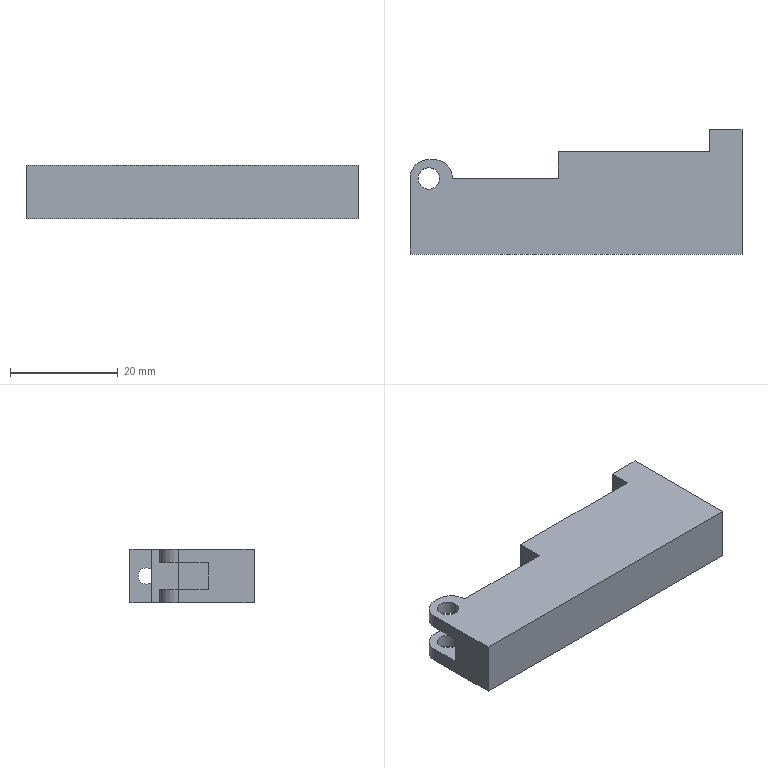Part | SolidWorks | features ICE 2, Extrusion 1 | 1 solid | 25 faces | box 61.5 x 23 x 10 mm | volume 10198 mm3 | plane 15 | cylinder 10 | commonest cylinder face diameters 4 x4 7 x4 3 x2
STEP:
#1=CARTESIAN_POINT('',(0.9754,7.251,6.5));
#2=VERTEX_POINT('',#1);
#3=CARTESIAN_POINT('',(0.9754,6.251,6.118));
#4=VERTEX_POINT('',#3);
#5=CARTESIAN_POINT('',(0.9754,7.251,5.));
#6=DIRECTION('',(1.,0.,0.));
#7=DIRECTION('',(0.,0.,-1.));
#8=AXIS2_PLACEMENT_3D('',#5,#6,#7);
#9=CIRCLE('',#8,1.5);
#10=EDGE_CURVE('',#2,#4,#9,.T.);
#11=ORIENTED_EDGE('',*,*,#10,.F.);
#12=CARTESIAN_POINT('',(6.975,7.251,6.5));
#13=VERTEX_POINT('',#12);
#14=CARTESIAN_POINT('',(0.9754,7.251,6.5));
#15=DIRECTION('',(1.,0.,0.));
#16=VECTOR('',#15,1000.);
#17=LINE('',#14,#16);
#18=EDGE_CURVE('',#2,#13,#17,.T.);
#19=ORIENTED_EDGE('',*,*,#18,.T.);
#20=CARTESIAN_POINT('',(6.975,7.251,3.5));
#21=VERTEX_POINT('',#20);
#22=CARTESIAN_POINT('',(6.975,7.251,5.));
#23=DIRECTION('',(1.,0.,0.));
#24=DIRECTION('',(0.,0.,-1.));
#25=AXIS2_PLACEMENT_3D('',#22,#23,#24);
#26=CIRCLE('',#25,1.5);
#27=EDGE_CURVE('',#13,#21,#26,.T.);
#28=ORIENTED_EDGE('',*,*,#27,.T.);
#29=CARTESIAN_POINT('',(0.9754,7.251,3.5));
#30=VERTEX_POINT('',#29);
#31=CARTESIAN_POINT('',(0.9754,7.251,3.5));
#32=DIRECTION('',(1.,0.,0.));
#33=VECTOR('',#32,1000.);
#34=LINE('',#31,#33);
#35=EDGE_CURVE('',#30,#21,#34,.T.);
#36=ORIENTED_EDGE('',*,*,#35,.F.);
#37=CARTESIAN_POINT('',(0.9754,6.251,3.882));
#38=VERTEX_POINT('',#37);
#39=CARTESIAN_POINT('',(0.9754,7.251,5.));
#40=DIRECTION('',(1.,0.,0.));
#41=DIRECTION('',(0.,0.,-1.));
#42=AXIS2_PLACEMENT_3D('',#39,#40,#41);
#43=CIRCLE('',#42,1.5);
#44=EDGE_CURVE('',#38,#30,#43,.T.);
#45=ORIENTED_EDGE('',*,*,#44,.F.);
#46=CARTESIAN_POINT('',(0.9754,7.251,5.));
#47=DIRECTION('',(1.,0.,0.));
#48=DIRECTION('',(0.,0.,-1.));
#49=AXIS2_PLACEMENT_3D('',#46,#47,#48);
#50=CIRCLE('',#49,1.5);
#51=EDGE_CURVE('',#4,#38,#50,.T.);
#52=ORIENTED_EDGE('',*,*,#51,.F.);
#53=EDGE_LOOP('',(#11,#19,#28,#36,#45,#52));
#54=FACE_OUTER_BOUND('',#53,.T.);
#55=CARTESIAN_POINT('',(0.9754,7.251,5.));
#56=DIRECTION('',(1.,0.,0.));
#57=DIRECTION('',(0.,0.,-1.));
#58=AXIS2_PLACEMENT_3D('',#55,#56,#57);
#59=CYLINDRICAL_SURFACE('',#58,1.5);
#60=ADVANCED_FACE('',(#54),#59,.F.);
#61=CARTESIAN_POINT('',(-49.025,1.251,2.5));
#62=VERTEX_POINT('',#61);
#63=CARTESIAN_POINT('',(-53.025,1.251,2.5));
#64=VERTEX_POINT('',#63);
#65=CARTESIAN_POINT('',(-51.025,1.251,2.5));
#66=DIRECTION('',(0.,0.,-1.));
#67=DIRECTION('',(0.,1.,0.));
#68=AXIS2_PLACEMENT_3D('',#65,#66,#67);
#69=CIRCLE('',#68,2.);
#70=EDGE_CURVE('',#62,#64,#69,.T.);
#71=ORIENTED_EDGE('',*,*,#70,.F.);
#72=CARTESIAN_POINT('',(-49.025,1.251,0.));
#73=VERTEX_POINT('',#72);
#74=CARTESIAN_POINT('',(-49.025,1.251,10.));
#75=DIRECTION('',(0.,0.,-1.));
#76=VECTOR('',#75,1000.);
#77=LINE('',#74,#76);
#78=EDGE_CURVE('',#62,#73,#77,.T.);
#79=ORIENTED_EDGE('',*,*,#78,.T.);
#80=CARTESIAN_POINT('',(-53.025,1.251,0.));
#81=VERTEX_POINT('',#80);
#82=CARTESIAN_POINT('',(-51.025,1.251,0.));
#83=DIRECTION('',(0.,0.,1.));
#84=DIRECTION('',(1.,0.,0.));
#85=AXIS2_PLACEMENT_3D('',#82,#83,#84);
#86=CIRCLE('',#85,2.);
#87=EDGE_CURVE('',#81,#73,#86,.T.);
#88=ORIENTED_EDGE('',*,*,#87,.F.);
#89=CARTESIAN_POINT('',(-53.025,1.251,10.));
#90=DIRECTION('',(0.,0.,-1.));
#91=VECTOR('',#90,1000.);
#92=LINE('',#89,#91);
#93=EDGE_CURVE('',#64,#81,#92,.T.);
#94=ORIENTED_EDGE('',*,*,#93,.F.);
#95=EDGE_LOOP('',(#71,#79,#88,#94));
#96=FACE_OUTER_BOUND('',#95,.T.);
#97=CARTESIAN_POINT('',(-51.025,1.251,10.));
#98=DIRECTION('',(0.,0.,-1.));
#99=DIRECTION('',(-1.,0.,0.));
#100=AXIS2_PLACEMENT_3D('',#97,#98,#99);
#101=CYLINDRICAL_SURFACE('',#100,2.);
#102=ADVANCED_FACE('',(#96),#101,.F.);
#103=CARTESIAN_POINT('',(-53.025,1.251,10.));
#104=VERTEX_POINT('',#103);
#105=CARTESIAN_POINT('',(-49.025,1.251,10.));
#106=VERTEX_POINT('',#105);
#107=CARTESIAN_POINT('',(-51.025,1.251,10.));
#108=DIRECTION('',(0.,0.,1.));
#109=DIRECTION('',(1.,0.,0.));
#110=AXIS2_PLACEMENT_3D('',#107,#108,#109);
#111=CIRCLE('',#110,2.);
#112=EDGE_CURVE('',#104,#106,#111,.T.);
#113=ORIENTED_EDGE('',*,*,#112,.T.);
#114=CARTESIAN_POINT('',(-49.025,1.251,7.5));
#115=VERTEX_POINT('',#114);
#116=CARTESIAN_POINT('',(-49.025,1.251,10.));
#117=DIRECTION('',(0.,0.,-1.));
#118=VECTOR('',#117,1000.);
#119=LINE('',#116,#118);
#120=EDGE_CURVE('',#106,#115,#119,.T.);
#121=ORIENTED_EDGE('',*,*,#120,.T.);
#122=CARTESIAN_POINT('',(-53.025,1.251,7.5));
#123=VERTEX_POINT('',#122);
#124=CARTESIAN_POINT('',(-51.025,1.251,7.5));
#125=DIRECTION('',(0.,0.,1.));
#126=DIRECTION('',(0.,-1.,0.));
#127=AXIS2_PLACEMENT_3D('',#124,#125,#126);
#128=CIRCLE('',#127,2.);
#129=EDGE_CURVE('',#123,#115,#128,.T.);
#130=ORIENTED_EDGE('',*,*,#129,.F.);
#131=CARTESIAN_POINT('',(-53.025,1.251,10.));
#132=DIRECTION('',(0.,0.,-1.));
#133=VECTOR('',#132,1000.);
#134=LINE('',#131,#133);
#135=EDGE_CURVE('',#104,#123,#134,.T.);
#136=ORIENTED_EDGE('',*,*,#135,.F.);
#137=EDGE_LOOP('',(#113,#121,#130,#136));
#138=FACE_OUTER_BOUND('',#137,.T.);
#139=CARTESIAN_POINT('',(-51.025,1.251,10.));
#140=DIRECTION('',(0.,0.,-1.));
#141=DIRECTION('',(-1.,0.,0.));
#142=AXIS2_PLACEMENT_3D('',#139,#140,#141);
#143=CYLINDRICAL_SURFACE('',#142,2.);
#144=ADVANCED_FACE('',(#138),#143,.F.);
#145=CARTESIAN_POINT('',(-50.595,4.725,2.5));
#146=VERTEX_POINT('',#145);
#147=CARTESIAN_POINT('',(-46.665,1.251,2.5));
#148=VERTEX_POINT('',#147);
#149=CARTESIAN_POINT('',(-50.165,1.251,2.5));
#150=DIRECTION('',(0.,0.,-1.));
#151=DIRECTION('',(0.,1.,0.));
#152=AXIS2_PLACEMENT_3D('',#149,#150,#151);
#153=CIRCLE('',#152,3.5);
#154=EDGE_CURVE('',#146,#148,#153,.T.);
#155=ORIENTED_EDGE('',*,*,#154,.T.);
#156=CARTESIAN_POINT('',(-46.665,1.251,0.));
#157=VERTEX_POINT('',#156);
#158=CARTESIAN_POINT('',(-46.665,1.251,10.));
#159=DIRECTION('',(0.,0.,-1.));
#160=VECTOR('',#159,1000.);
#161=LINE('',#158,#160);
#162=EDGE_CURVE('',#148,#157,#161,.T.);
#163=ORIENTED_EDGE('',*,*,#162,.T.);
#164=CARTESIAN_POINT('',(-50.595,4.725,0.));
#165=VERTEX_POINT('',#164);
#166=CARTESIAN_POINT('',(-50.165,1.251,0.));
#167=DIRECTION('',(0.,0.,1.));
#168=DIRECTION('',(1.,0.,0.));
#169=AXIS2_PLACEMENT_3D('',#166,#167,#168);
#170=CIRCLE('',#169,3.5);
#171=EDGE_CURVE('',#157,#165,#170,.T.);
#172=ORIENTED_EDGE('',*,*,#171,.T.);
#173=CARTESIAN_POINT('',(-50.595,4.725,10.));
#174=DIRECTION('',(0.,0.,-1.));
#175=VECTOR('',#174,1000.);
#176=LINE('',#173,#175);
#177=EDGE_CURVE('',#146,#165,#176,.T.);
#178=ORIENTED_EDGE('',*,*,#177,.F.);
#179=EDGE_LOOP('',(#155,#163,#172,#178));
#180=FACE_OUTER_BOUND('',#179,.T.);
#181=CARTESIAN_POINT('',(-50.165,1.251,10.));
#182=DIRECTION('',(0.,0.,-1.));
#183=DIRECTION('',(-1.,0.,0.));
#184=AXIS2_PLACEMENT_3D('',#181,#182,#183);
#185=CYLINDRICAL_SURFACE('',#184,3.5);
#186=ADVANCED_FACE('',(#180),#185,.T.);
#187=CARTESIAN_POINT('',(-54.525,1.251,2.5));
#188=VERTEX_POINT('',#187);
#189=CARTESIAN_POINT('',(-51.025,1.251,2.5));
#190=DIRECTION('',(0.,0.,-1.));
#191=DIRECTION('',(0.,1.,0.));
#192=AXIS2_PLACEMENT_3D('',#189,#190,#191);
#193=CIRCLE('',#192,3.5);
#194=EDGE_CURVE('',#188,#146,#193,.T.);
#195=ORIENTED_EDGE('',*,*,#194,.T.);
#196=ORIENTED_EDGE('',*,*,#177,.T.);
#197=CARTESIAN_POINT('',(-54.525,1.251,0.));
#198=VERTEX_POINT('',#197);
#199=CARTESIAN_POINT('',(-51.025,1.251,0.));
#200=DIRECTION('',(0.,0.,1.));
#201=DIRECTION('',(1.,0.,0.));
#202=AXIS2_PLACEMENT_3D('',#199,#200,#201);
#203=CIRCLE('',#202,3.5);
#204=EDGE_CURVE('',#165,#198,#203,.T.);
#205=ORIENTED_EDGE('',*,*,#204,.T.);
#206=CARTESIAN_POINT('',(-54.525,1.251,10.));
#207=DIRECTION('',(0.,0.,-1.));
#208=VECTOR('',#207,1000.);
#209=LINE('',#206,#208);
#210=EDGE_CURVE('',#188,#198,#209,.T.);
#211=ORIENTED_EDGE('',*,*,#210,.F.);
#212=EDGE_LOOP('',(#195,#196,#205,#211));
#213=FACE_OUTER_BOUND('',#212,.T.);
#214=CARTESIAN_POINT('',(-51.025,1.251,10.));
#215=DIRECTION('',(0.,0.,-1.));
#216=DIRECTION('',(-1.,0.,0.));
#217=AXIS2_PLACEMENT_3D('',#214,#215,#216);
#218=CYLINDRICAL_SURFACE('',#217,3.5);
#219=ADVANCED_FACE('',(#213),#218,.T.);
#220=ORIENTED_EDGE('',*,*,#120,.F.);
#221=CARTESIAN_POINT('',(-51.025,1.251,10.));
#222=DIRECTION('',(0.,0.,1.));
#223=DIRECTION('',(1.,0.,0.));
#224=AXIS2_PLACEMENT_3D('',#221,#222,#223);
#225=CIRCLE('',#224,2.);
#226=EDGE_CURVE('',#106,#104,#225,.T.);
#227=ORIENTED_EDGE('',*,*,#226,.T.);
#228=ORIENTED_EDGE('',*,*,#135,.T.);
#229=CARTESIAN_POINT('',(-51.025,1.251,7.5));
#230=DIRECTION('',(0.,0.,1.));
#231=DIRECTION('',(0.,-1.,0.));
#232=AXIS2_PLACEMENT_3D('',#229,#230,#231);
#233=CIRCLE('',#232,2.);
#234=EDGE_CURVE('',#115,#123,#233,.T.);
#235=ORIENTED_EDGE('',*,*,#234,.F.);
#236=EDGE_LOOP('',(#220,#227,#228,#235));
#237=FACE_OUTER_BOUND('',#236,.T.);
#238=CARTESIAN_POINT('',(-51.025,1.251,10.));
#239=DIRECTION('',(0.,0.,-1.));
#240=DIRECTION('',(-1.,0.,0.));
#241=AXIS2_PLACEMENT_3D('',#238,#239,#240);
#242=CYLINDRICAL_SURFACE('',#241,2.);
#243=ADVANCED_FACE('',(#237),#242,.F.);
#244=CARTESIAN_POINT('',(-46.665,1.251,7.5));
#245=VERTEX_POINT('',#244);
#246=CARTESIAN_POINT('',(-41.525,1.251,7.5));
#247=VERTEX_POINT('',#246);
#248=CARTESIAN_POINT('',(0.,1.251,7.5));
#249=DIRECTION('',(1.,0.,0.));
#250=VECTOR('',#249,1000.);
#251=LINE('',#248,#250);
#252=EDGE_CURVE('',#245,#247,#251,.T.);
#253=ORIENTED_EDGE('',*,*,#252,.F.);
#254=CARTESIAN_POINT('',(-46.665,1.251,10.));
#255=VERTEX_POINT('',#254);
#256=CARTESIAN_POINT('',(-46.665,1.251,10.));
#257=DIRECTION('',(0.,0.,-1.));
#258=VECTOR('',#257,1000.);
#259=LINE('',#256,#258);
#260=EDGE_CURVE('',#255,#245,#259,.T.);
#261=ORIENTED_EDGE('',*,*,#260,.F.);
#262=CARTESIAN_POINT('',(-27.025,1.251,10.));
#263=VERTEX_POINT('',#262);
#264=CARTESIAN_POINT('',(0.,1.251,10.));
#265=DIRECTION('',(1.,0.,0.));
#266=VECTOR('',#265,1000.);
#267=LINE('',#264,#266);
#268=EDGE_CURVE('',#255,#263,#267,.T.);
#269=ORIENTED_EDGE('',*,*,#268,.T.);
#270=CARTESIAN_POINT('',(-27.025,1.251,0.));
#271=VERTEX_POINT('',#270);
#272=CARTESIAN_POINT('',(-27.025,1.251,10.));
#273=DIRECTION('',(0.,0.,-1.));
#274=VECTOR('',#273,1000.);
#275=LINE('',#272,#274);
#276=EDGE_CURVE('',#263,#271,#275,.T.);
#277=ORIENTED_EDGE('',*,*,#276,.T.);
#278=CARTESIAN_POINT('',(0.,1.251,0.));
#279=DIRECTION('',(1.,0.,0.));
#280=VECTOR('',#279,1000.);
#281=LINE('',#278,#280);
#282=EDGE_CURVE('',#157,#271,#281,.T.);
#283=ORIENTED_EDGE('',*,*,#282,.F.);
#284=ORIENTED_EDGE('',*,*,#162,.F.);
#285=CARTESIAN_POINT('',(-41.525,1.251,2.5));
#286=VERTEX_POINT('',#285);
#287=CARTESIAN_POINT('',(0.,1.251,2.5));
#288=DIRECTION('',(-1.,0.,0.));
#289=VECTOR('',#288,1000.);
#290=LINE('',#287,#289);
#291=EDGE_CURVE('',#286,#148,#290,.T.);
#292=ORIENTED_EDGE('',*,*,#291,.F.);
#293=CARTESIAN_POINT('',(-41.525,1.251,10.));
#294=DIRECTION('',(0.,0.,-1.));
#295=VECTOR('',#294,1000.);
#296=LINE('',#293,#295);
#297=EDGE_CURVE('',#247,#286,#296,.T.);
#298=ORIENTED_EDGE('',*,*,#297,.F.);
#299=EDGE_LOOP('',(#253,#261,#269,#277,#283,#284,#292,#298));
#300=FACE_OUTER_BOUND('',#299,.T.);
#301=CARTESIAN_POINT('',(0.,1.251,10.));
#302=DIRECTION('',(0.,1.,0.));
#303=DIRECTION('',(0.,0.,1.));
#304=AXIS2_PLACEMENT_3D('',#301,#302,#303);
#305=PLANE('',#304);
#306=ADVANCED_FACE('',(#300),#305,.T.);
#307=CARTESIAN_POINT('',(-50.595,4.725,7.5));
#308=VERTEX_POINT('',#307);
#309=CARTESIAN_POINT('',(-50.165,1.251,7.5));
#310=DIRECTION('',(0.,0.,1.));
#311=DIRECTION('',(0.,-1.,0.));
#312=AXIS2_PLACEMENT_3D('',#309,#310,#311);
#313=CIRCLE('',#312,3.5);
#314=EDGE_CURVE('',#245,#308,#313,.T.);
#315=ORIENTED_EDGE('',*,*,#314,.T.);
#316=CARTESIAN_POINT('',(-50.595,4.725,10.));
#317=VERTEX_POINT('',#316);
#318=CARTESIAN_POINT('',(-50.595,4.725,10.));
#319=DIRECTION('',(0.,0.,-1.));
#320=VECTOR('',#319,1000.);
#321=LINE('',#318,#320);
#322=EDGE_CURVE('',#317,#308,#321,.T.);
#323=ORIENTED_EDGE('',*,*,#322,.F.);
#324=CARTESIAN_POINT('',(-50.165,1.251,10.));
#325=DIRECTION('',(0.,0.,1.));
#326=DIRECTION('',(1.,0.,0.));
#327=AXIS2_PLACEMENT_3D('',#324,#325,#326);
#328=CIRCLE('',#327,3.5);
#329=EDGE_CURVE('',#255,#317,#328,.T.);
#330=ORIENTED_EDGE('',*,*,#329,.F.);
#331=ORIENTED_EDGE('',*,*,#260,.T.);
#332=EDGE_LOOP('',(#315,#323,#330,#331));
#333=FACE_OUTER_BOUND('',#332,.T.);
#334=CARTESIAN_POINT('',(-50.165,1.251,10.));
#335=DIRECTION('',(0.,0.,-1.));
#336=DIRECTION('',(-1.,0.,0.));
#337=AXIS2_PLACEMENT_3D('',#334,#335,#336);
#338=CYLINDRICAL_SURFACE('',#337,3.5);
#339=ADVANCED_FACE('',(#333),#338,.T.);
#340=CARTESIAN_POINT('',(-54.525,1.251,7.5));
#341=VERTEX_POINT('',#340);
#342=CARTESIAN_POINT('',(-51.025,1.251,7.5));
#343=DIRECTION('',(0.,0.,1.));
#344=DIRECTION('',(0.,-1.,0.));
#345=AXIS2_PLACEMENT_3D('',#342,#343,#344);
#346=CIRCLE('',#345,3.5);
#347=EDGE_CURVE('',#308,#341,#346,.T.);
#348=ORIENTED_EDGE('',*,*,#347,.T.);
#349=CARTESIAN_POINT('',(-54.525,1.251,10.));
#350=VERTEX_POINT('',#349);
#351=CARTESIAN_POINT('',(-54.525,1.251,10.));
#352=DIRECTION('',(0.,0.,-1.));
#353=VECTOR('',#352,1000.);
#354=LINE('',#351,#353);
#355=EDGE_CURVE('',#350,#341,#354,.T.);
#356=ORIENTED_EDGE('',*,*,#355,.F.);
#357=CARTESIAN_POINT('',(-51.025,1.251,10.));
#358=DIRECTION('',(0.,0.,1.));
#359=DIRECTION('',(1.,0.,0.));
#360=AXIS2_PLACEMENT_3D('',#357,#358,#359);
#361=CIRCLE('',#360,3.5);
#362=EDGE_CURVE('',#317,#350,#361,.T.);
#363=ORIENTED_EDGE('',*,*,#362,.F.);
#364=ORIENTED_EDGE('',*,*,#322,.T.);
#365=EDGE_LOOP('',(#348,#356,#363,#364));
#366=FACE_OUTER_BOUND('',#365,.T.);
#367=CARTESIAN_POINT('',(-51.025,1.251,10.));
#368=DIRECTION('',(0.,0.,-1.));
#369=DIRECTION('',(-1.,0.,0.));
#370=AXIS2_PLACEMENT_3D('',#367,#368,#369);
#371=CYLINDRICAL_SURFACE('',#370,3.5);
#372=ADVANCED_FACE('',(#366),#371,.T.);
#373=ORIENTED_EDGE('',*,*,#355,.T.);
#374=CARTESIAN_POINT('',(-54.525,-4.249,7.5));
#375=VERTEX_POINT('',#374);
#376=CARTESIAN_POINT('',(-54.525,-4.249,7.5));
#377=DIRECTION('',(0.,1.,0.));
#378=VECTOR('',#377,1000.);
#379=LINE('',#376,#378);
#380=EDGE_CURVE('',#375,#341,#379,.T.);
#381=ORIENTED_EDGE('',*,*,#380,.F.);
#382=CARTESIAN_POINT('',(-54.525,-4.249,2.5));
#383=VERTEX_POINT('',#382);
#384=CARTESIAN_POINT('',(-54.525,-4.249,2.5));
#385=DIRECTION('',(0.,0.,1.));
#386=VECTOR('',#385,1000.);
#387=LINE('',#384,#386);
#388=EDGE_CURVE('',#383,#375,#387,.T.);
#389=ORIENTED_EDGE('',*,*,#388,.F.);
#390=CARTESIAN_POINT('',(-54.525,4.751,2.5));
#391=DIRECTION('',(0.,-1.,0.));
#392=VECTOR('',#391,1000.);
#393=LINE('',#390,#392);
#394=EDGE_CURVE('',#188,#383,#393,.T.);
#395=ORIENTED_EDGE('',*,*,#394,.F.);
#396=ORIENTED_EDGE('',*,*,#210,.T.);
#397=CARTESIAN_POINT('',(-54.525,-12.749,0.));
#398=VERTEX_POINT('',#397);
#399=CARTESIAN_POINT('',(-54.525,0.,0.));
#400=DIRECTION('',(0.,-1.,0.));
#401=VECTOR('',#400,1000.);
#402=LINE('',#399,#401);
#403=EDGE_CURVE('',#198,#398,#402,.T.);
#404=ORIENTED_EDGE('',*,*,#403,.T.);
#405=CARTESIAN_POINT('',(-54.525,-12.749,10.));
#406=VERTEX_POINT('',#405);
#407=CARTESIAN_POINT('',(-54.525,-12.749,10.));
#408=DIRECTION('',(0.,0.,-1.));
#409=VECTOR('',#408,1000.);
#410=LINE('',#407,#409);
#411=EDGE_CURVE('',#406,#398,#410,.T.);
#412=ORIENTED_EDGE('',*,*,#411,.F.);
#413=CARTESIAN_POINT('',(-54.525,0.,10.));
#414=DIRECTION('',(0.,-1.,0.));
#415=VECTOR('',#414,1000.);
#416=LINE('',#413,#415);
#417=EDGE_CURVE('',#350,#406,#416,.T.);
#418=ORIENTED_EDGE('',*,*,#417,.F.);
#419=EDGE_LOOP('',(#373,#381,#389,#395,#396,#404,#412,#418));
#420=FACE_OUTER_BOUND('',#419,.T.);
#421=CARTESIAN_POINT('',(-54.525,0.,10.));
#422=DIRECTION('',(1.,0.,0.));
#423=DIRECTION('',(0.,0.,-1.));
#424=AXIS2_PLACEMENT_3D('',#421,#422,#423);
#425=PLANE('',#424);
#426=ADVANCED_FACE('',(#420),#425,.F.);
#427=CARTESIAN_POINT('',(6.975,-12.749,0.));
#428=VERTEX_POINT('',#427);
#429=CARTESIAN_POINT('',(0.,-12.749,0.));
#430=DIRECTION('',(-1.,0.,0.));
#431=VECTOR('',#430,1000.);
#432=LINE('',#429,#431);
#433=EDGE_CURVE('',#428,#398,#432,.T.);
#434=ORIENTED_EDGE('',*,*,#433,.F.);
#435=CARTESIAN_POINT('',(6.975,-12.749,10.));
#436=VERTEX_POINT('',#435);
#437=CARTESIAN_POINT('',(6.975,-12.749,10.));
#438=DIRECTION('',(0.,0.,-1.));
#439=VECTOR('',#438,1000.);
#440=LINE('',#437,#439);
#441=EDGE_CURVE('',#436,#428,#440,.T.);
#442=ORIENTED_EDGE('',*,*,#441,.F.);
#443=CARTESIAN_POINT('',(0.,-12.749,10.));
#444=DIRECTION('',(-1.,0.,0.));
#445=VECTOR('',#444,1000.);
#446=LINE('',#443,#445);
#447=EDGE_CURVE('',#436,#406,#446,.T.);
#448=ORIENTED_EDGE('',*,*,#447,.T.);
#449=ORIENTED_EDGE('',*,*,#411,.T.);
#450=EDGE_LOOP('',(#434,#442,#448,#449));
#451=FACE_OUTER_BOUND('',#450,.T.);
#452=CARTESIAN_POINT('',(0.,-12.749,10.));
#453=DIRECTION('',(0.,-1.,0.));
#454=DIRECTION('',(1.,0.,0.));
#455=AXIS2_PLACEMENT_3D('',#452,#453,#454);
#456=PLANE('',#455);
#457=ADVANCED_FACE('',(#451),#456,.T.);
#458=CARTESIAN_POINT('',(6.975,7.251,5.));
#459=DIRECTION('',(1.,0.,0.));
#460=DIRECTION('',(0.,0.,-1.));
#461=AXIS2_PLACEMENT_3D('',#458,#459,#460);
#462=CIRCLE('',#461,1.5);
#463=EDGE_CURVE('',#21,#13,#462,.T.);
#464=ORIENTED_EDGE('',*,*,#463,.F.);
#465=ORIENTED_EDGE('',*,*,#27,.F.);
#466=EDGE_LOOP('',(#464,#465));
#467=FACE_BOUND('',#466,.T.);
#468=CARTESIAN_POINT('',(6.975,10.251,0.));
#469=VERTEX_POINT('',#468);
#470=CARTESIAN_POINT('',(6.975,0.,0.));
#471=DIRECTION('',(0.,-1.,0.));
#472=VECTOR('',#471,1000.);
#473=LINE('',#470,#472);
#474=EDGE_CURVE('',#469,#428,#473,.T.);
#475=ORIENTED_EDGE('',*,*,#474,.F.);
#476=CARTESIAN_POINT('',(6.975,10.251,10.));
#477=VERTEX_POINT('',#476);
#478=CARTESIAN_POINT('',(6.975,10.251,10.));
#479=DIRECTION('',(0.,0.,-1.));
#480=VECTOR('',#479,1000.);
#481=LINE('',#478,#480);
#482=EDGE_CURVE('',#477,#469,#481,.T.);
#483=ORIENTED_EDGE('',*,*,#482,.F.);
#484=CARTESIAN_POINT('',(6.975,0.,10.));
#485=DIRECTION('',(0.,-1.,0.));
#486=VECTOR('',#485,1000.);
#487=LINE('',#484,#486);
#488=EDGE_CURVE('',#477,#436,#487,.T.);
#489=ORIENTED_EDGE('',*,*,#488,.T.);
#490=ORIENTED_EDGE('',*,*,#441,.T.);
#491=EDGE_LOOP('',(#475,#483,#489,#490));
#492=FACE_OUTER_BOUND('',#491,.T.);
#493=CARTESIAN_POINT('',(6.975,0.,10.));
#494=DIRECTION('',(1.,0.,0.));
#495=DIRECTION('',(0.,0.,-1.));
#496=AXIS2_PLACEMENT_3D('',#493,#494,#495);
#497=PLANE('',#496);
#498=ADVANCED_FACE('',(#467,#492),#497,.T.);
#499=CARTESIAN_POINT('',(0.9754,10.251,0.));
#500=VERTEX_POINT('',#499);
#501=CARTESIAN_POINT('',(0.,10.251,0.));
#502=DIRECTION('',(1.,0.,0.));
#503=VECTOR('',#502,1000.);
#504=LINE('',#501,#503);
#505=EDGE_CURVE('',#500,#469,#504,.T.);
#506=ORIENTED_EDGE('',*,*,#505,.F.);
#507=CARTESIAN_POINT('',(0.9754,10.251,10.));
#508=VERTEX_POINT('',#507);
#509=CARTESIAN_POINT('',(0.9754,10.251,10.));
#510=DIRECTION('',(0.,0.,-1.));
#511=VECTOR('',#510,1000.);
#512=LINE('',#509,#511);
#513=EDGE_CURVE('',#508,#500,#512,.T.);
#514=ORIENTED_EDGE('',*,*,#513,.F.);
#515=CARTESIAN_POINT('',(0.,10.251,10.));
#516=DIRECTION('',(1.,0.,0.));
#517=VECTOR('',#516,1000.);
#518=LINE('',#515,#517);
#519=EDGE_CURVE('',#508,#477,#518,.T.);
#520=ORIENTED_EDGE('',*,*,#519,.T.);
#521=ORIENTED_EDGE('',*,*,#482,.T.);
#522=EDGE_LOOP('',(#506,#514,#520,#521));
#523=FACE_OUTER_BOUND('',#522,.T.);
#524=CARTESIAN_POINT('',(0.,10.251,10.));
#525=DIRECTION('',(0.,1.,0.));
#526=DIRECTION('',(0.,0.,1.));
#527=AXIS2_PLACEMENT_3D('',#524,#525,#526);
#528=PLANE('',#527);
#529=ADVANCED_FACE('',(#523),#528,.T.);
#530=ORIENTED_EDGE('',*,*,#44,.T.);
#531=CARTESIAN_POINT('',(0.9754,7.251,5.));
#532=DIRECTION('',(1.,0.,0.));
#533=DIRECTION('',(0.,0.,-1.));
#534=AXIS2_PLACEMENT_3D('',#531,#532,#533);
#535=CIRCLE('',#534,1.5);
#536=EDGE_CURVE('',#30,#2,#535,.T.);
#537=ORIENTED_EDGE('',*,*,#536,.T.);
#538=ORIENTED_EDGE('',*,*,#10,.T.);
#539=CARTESIAN_POINT('',(0.9754,6.251,10.));
#540=VERTEX_POINT('',#539);
#541=CARTESIAN_POINT('',(0.9754,6.251,10.));
#542=DIRECTION('',(0.,0.,-1.));
#543=VECTOR('',#542,1000.);
#544=LINE('',#541,#543);
#545=EDGE_CURVE('',#540,#4,#544,.T.);
#546=ORIENTED_EDGE('',*,*,#545,.F.);
#547=CARTESIAN_POINT('',(0.9754,0.,10.));
#548=DIRECTION('',(0.,1.,0.));
#549=VECTOR('',#548,1000.);
#550=LINE('',#547,#549);
#551=EDGE_CURVE('',#540,#508,#550,.T.);
#552=ORIENTED_EDGE('',*,*,#551,.T.);
#553=ORIENTED_EDGE('',*,*,#513,.T.);
#554=CARTESIAN_POINT('',(0.9754,6.251,0.));
#555=VERTEX_POINT('',#554);
#556=CARTESIAN_POINT('',(0.9754,0.,0.));
#557=DIRECTION('',(0.,1.,0.));
#558=VECTOR('',#557,1000.);
#559=LINE('',#556,#558);
#560=EDGE_CURVE('',#555,#500,#559,.T.);
#561=ORIENTED_EDGE('',*,*,#560,.F.);
#562=CARTESIAN_POINT('',(0.9754,6.251,10.));
#563=DIRECTION('',(0.,0.,-1.));
#564=VECTOR('',#563,1000.);
#565=LINE('',#562,#564);
#566=EDGE_CURVE('',#38,#555,#565,.T.);
#567=ORIENTED_EDGE('',*,*,#566,.F.);
#568=EDGE_LOOP('',(#530,#537,#538,#546,#552,#553,#561,#567));
#569=FACE_OUTER_BOUND('',#568,.T.);
#570=CARTESIAN_POINT('',(0.9754,0.,10.));
#571=DIRECTION('',(-1.,0.,0.));
#572=DIRECTION('',(0.,0.,1.));
#573=AXIS2_PLACEMENT_3D('',#570,#571,#572);
#574=PLANE('',#573);
#575=ADVANCED_FACE('',(#569),#574,.T.);
#576=CARTESIAN_POINT('',(-27.025,6.251,0.));
#577=VERTEX_POINT('',#576);
#578=CARTESIAN_POINT('',(0.,6.251,0.));
#579=DIRECTION('',(1.,0.,0.));
#580=VECTOR('',#579,1000.);
#581=LINE('',#578,#580);
#582=EDGE_CURVE('',#577,#555,#581,.T.);
#583=ORIENTED_EDGE('',*,*,#582,.F.);
#584=CARTESIAN_POINT('',(-27.025,6.251,10.));
#585=VERTEX_POINT('',#584);
#586=CARTESIAN_POINT('',(-27.025,6.251,10.));
#587=DIRECTION('',(0.,0.,-1.));
#588=VECTOR('',#587,1000.);
#589=LINE('',#586,#588);
#590=EDGE_CURVE('',#585,#577,#589,.T.);
#591=ORIENTED_EDGE('',*,*,#590,.F.);
#592=CARTESIAN_POINT('',(0.,6.251,10.));
#593=DIRECTION('',(1.,0.,0.));
#594=VECTOR('',#593,1000.);
#595=LINE('',#592,#594);
#596=EDGE_CURVE('',#585,#540,#595,.T.);
#597=ORIENTED_EDGE('',*,*,#596,.T.);
#598=ORIENTED_EDGE('',*,*,#545,.T.);
#599=CARTESIAN_POINT('',(0.9754,6.251,10.));
#600=DIRECTION('',(0.,0.,-1.));
#601=VECTOR('',#600,1000.);
#602=LINE('',#599,#601);
#603=EDGE_CURVE('',#4,#38,#602,.T.);
#604=ORIENTED_EDGE('',*,*,#603,.T.);
#605=ORIENTED_EDGE('',*,*,#566,.T.);
#606=EDGE_LOOP('',(#583,#591,#597,#598,#604,#605));
#607=FACE_OUTER_BOUND('',#606,.T.);
#608=CARTESIAN_POINT('',(0.,6.251,10.));
#609=DIRECTION('',(0.,1.,0.));
#610=DIRECTION('',(0.,0.,1.));
#611=AXIS2_PLACEMENT_3D('',#608,#609,#610);
#612=PLANE('',#611);
#613=ADVANCED_FACE('',(#607),#612,.T.);
#614=ORIENTED_EDGE('',*,*,#78,.F.);
#615=CARTESIAN_POINT('',(-51.025,1.251,2.5));
#616=DIRECTION('',(0.,0.,-1.));
#617=DIRECTION('',(0.,1.,0.));
#618=AXIS2_PLACEMENT_3D('',#615,#616,#617);
#619=CIRCLE('',#618,2.);
#620=EDGE_CURVE('',#64,#62,#619,.T.);
#621=ORIENTED_EDGE('',*,*,#620,.F.);
#622=ORIENTED_EDGE('',*,*,#93,.T.);
#623=CARTESIAN_POINT('',(-51.025,1.251,0.));
#624=DIRECTION('',(0.,0.,1.));
#625=DIRECTION('',(1.,0.,0.));
#626=AXIS2_PLACEMENT_3D('',#623,#624,#625);
#627=CIRCLE('',#626,2.);
#628=EDGE_CURVE('',#73,#81,#627,.T.);
#629=ORIENTED_EDGE('',*,*,#628,.F.);
#630=EDGE_LOOP('',(#614,#621,#622,#629));
#631=FACE_OUTER_BOUND('',#630,.T.);
#632=CARTESIAN_POINT('',(-51.025,1.251,10.));
#633=DIRECTION('',(0.,0.,-1.));
#634=DIRECTION('',(-1.,0.,0.));
#635=AXIS2_PLACEMENT_3D('',#632,#633,#634);
#636=CYLINDRICAL_SURFACE('',#635,2.);
#637=ADVANCED_FACE('',(#631),#636,.F.);
#638=CARTESIAN_POINT('',(-27.025,0.,0.));
#639=DIRECTION('',(0.,1.,0.));
#640=VECTOR('',#639,1000.);
#641=LINE('',#638,#640);
#642=EDGE_CURVE('',#271,#577,#641,.T.);
#643=ORIENTED_EDGE('',*,*,#642,.F.);
#644=ORIENTED_EDGE('',*,*,#276,.F.);
#645=CARTESIAN_POINT('',(-27.025,0.,10.));
#646=DIRECTION('',(0.,1.,0.));
#647=VECTOR('',#646,1000.);
#648=LINE('',#645,#647);
#649=EDGE_CURVE('',#263,#585,#648,.T.);
#650=ORIENTED_EDGE('',*,*,#649,.T.);
#651=ORIENTED_EDGE('',*,*,#590,.T.);
#652=EDGE_LOOP('',(#643,#644,#650,#651));
#653=FACE_OUTER_BOUND('',#652,.T.);
#654=CARTESIAN_POINT('',(-27.025,0.,10.));
#655=DIRECTION('',(-1.,0.,0.));
#656=DIRECTION('',(0.,0.,1.));
#657=AXIS2_PLACEMENT_3D('',#654,#655,#656);
#658=PLANE('',#657);
#659=ADVANCED_FACE('',(#653),#658,.T.);
#660=ORIENTED_EDGE('',*,*,#112,.F.);
#661=ORIENTED_EDGE('',*,*,#226,.F.);
#662=EDGE_LOOP('',(#660,#661));
#663=FACE_BOUND('',#662,.T.);
#664=ORIENTED_EDGE('',*,*,#268,.F.);
#665=ORIENTED_EDGE('',*,*,#329,.T.);
#666=ORIENTED_EDGE('',*,*,#362,.T.);
#667=ORIENTED_EDGE('',*,*,#417,.T.);
#668=ORIENTED_EDGE('',*,*,#447,.F.);
#669=ORIENTED_EDGE('',*,*,#488,.F.);
#670=ORIENTED_EDGE('',*,*,#519,.F.);
#671=ORIENTED_EDGE('',*,*,#551,.F.);
#672=ORIENTED_EDGE('',*,*,#596,.F.);
#673=ORIENTED_EDGE('',*,*,#649,.F.);
#674=EDGE_LOOP('',(#664,#665,#666,#667,#668,#669,#670,#671,#672,#673));
#675=FACE_OUTER_BOUND('',#674,.T.);
#676=CARTESIAN_POINT('',(0.,0.,10.));
#677=DIRECTION('',(0.,0.,1.));
#678=DIRECTION('',(1.,0.,0.));
#679=AXIS2_PLACEMENT_3D('',#676,#677,#678);
#680=PLANE('',#679);
#681=ADVANCED_FACE('',(#663,#675),#680,.T.);
#682=ORIENTED_EDGE('',*,*,#87,.T.);
#683=ORIENTED_EDGE('',*,*,#628,.T.);
#684=EDGE_LOOP('',(#682,#683));
#685=FACE_BOUND('',#684,.T.);
#686=ORIENTED_EDGE('',*,*,#282,.T.);
#687=ORIENTED_EDGE('',*,*,#642,.T.);
#688=ORIENTED_EDGE('',*,*,#582,.T.);
#689=ORIENTED_EDGE('',*,*,#560,.T.);
#690=ORIENTED_EDGE('',*,*,#505,.T.);
#691=ORIENTED_EDGE('',*,*,#474,.T.);
#692=ORIENTED_EDGE('',*,*,#433,.T.);
#693=ORIENTED_EDGE('',*,*,#403,.F.);
#694=ORIENTED_EDGE('',*,*,#204,.F.);
#695=ORIENTED_EDGE('',*,*,#171,.F.);
#696=EDGE_LOOP('',(#686,#687,#688,#689,#690,#691,#692,#693,#694,#695));
#697=FACE_OUTER_BOUND('',#696,.T.);
#698=CARTESIAN_POINT('',(0.,0.,0.));
#699=DIRECTION('',(0.,0.,1.));
#700=DIRECTION('',(1.,0.,0.));
#701=AXIS2_PLACEMENT_3D('',#698,#699,#700);
#702=PLANE('',#701);
#703=ADVANCED_FACE('',(#685,#697),#702,.F.);
#704=ORIENTED_EDGE('',*,*,#18,.F.);
#705=ORIENTED_EDGE('',*,*,#536,.F.);
#706=ORIENTED_EDGE('',*,*,#35,.T.);
#707=ORIENTED_EDGE('',*,*,#463,.T.);
#708=EDGE_LOOP('',(#704,#705,#706,#707));
#709=FACE_OUTER_BOUND('',#708,.T.);
#710=CARTESIAN_POINT('',(0.9754,7.251,5.));
#711=DIRECTION('',(1.,0.,0.));
#712=DIRECTION('',(0.,0.,-1.));
#713=AXIS2_PLACEMENT_3D('',#710,#711,#712);
#714=CYLINDRICAL_SURFACE('',#713,1.5);
#715=ADVANCED_FACE('',(#709),#714,.F.);
#716=ORIENTED_EDGE('',*,*,#51,.T.);
#717=ORIENTED_EDGE('',*,*,#603,.F.);
#718=EDGE_LOOP('',(#716,#717));
#719=FACE_OUTER_BOUND('',#718,.T.);
#720=CARTESIAN_POINT('',(0.9754,7.251,5.));
#721=DIRECTION('',(1.,0.,0.));
#722=DIRECTION('',(0.,0.,-1.));
#723=AXIS2_PLACEMENT_3D('',#720,#721,#722);
#724=PLANE('',#723);
#725=ADVANCED_FACE('',(#719),#724,.T.);
#726=ORIENTED_EDGE('',*,*,#252,.T.);
#727=CARTESIAN_POINT('',(-41.525,-4.249,7.5));
#728=VERTEX_POINT('',#727);
#729=CARTESIAN_POINT('',(-41.525,-4.249,7.5));
#730=DIRECTION('',(0.,1.,0.));
#731=VECTOR('',#730,1000.);
#732=LINE('',#729,#731);
#733=EDGE_CURVE('',#728,#247,#732,.T.);
#734=ORIENTED_EDGE('',*,*,#733,.F.);
#735=CARTESIAN_POINT('',(-41.525,-4.249,7.5));
#736=DIRECTION('',(-1.,0.,0.));
#737=VECTOR('',#736,1000.);
#738=LINE('',#735,#737);
#739=EDGE_CURVE('',#728,#375,#738,.T.);
#740=ORIENTED_EDGE('',*,*,#739,.T.);
#741=ORIENTED_EDGE('',*,*,#380,.T.);
#742=ORIENTED_EDGE('',*,*,#347,.F.);
#743=ORIENTED_EDGE('',*,*,#314,.F.);
#744=EDGE_LOOP('',(#726,#734,#740,#741,#742,#743));
#745=FACE_OUTER_BOUND('',#744,.T.);
#746=ORIENTED_EDGE('',*,*,#129,.T.);
#747=ORIENTED_EDGE('',*,*,#234,.T.);
#748=EDGE_LOOP('',(#746,#747));
#749=FACE_BOUND('',#748,.T.);
#750=CARTESIAN_POINT('',(-41.525,-4.249,7.5));
#751=DIRECTION('',(0.,0.,1.));
#752=DIRECTION('',(0.,-1.,0.));
#753=AXIS2_PLACEMENT_3D('',#750,#751,#752);
#754=PLANE('',#753);
#755=ADVANCED_FACE('',(#745,#749),#754,.F.);
#756=ORIENTED_EDGE('',*,*,#291,.T.);
#757=ORIENTED_EDGE('',*,*,#154,.F.);
#758=ORIENTED_EDGE('',*,*,#194,.F.);
#759=ORIENTED_EDGE('',*,*,#394,.T.);
#760=CARTESIAN_POINT('',(-41.525,-4.249,2.5));
#761=VERTEX_POINT('',#760);
#762=CARTESIAN_POINT('',(-41.525,-4.249,2.5));
#763=DIRECTION('',(-1.,0.,0.));
#764=VECTOR('',#763,1000.);
#765=LINE('',#762,#764);
#766=EDGE_CURVE('',#761,#383,#765,.T.);
#767=ORIENTED_EDGE('',*,*,#766,.F.);
#768=CARTESIAN_POINT('',(-41.525,4.751,2.5));
#769=DIRECTION('',(0.,-1.,0.));
#770=VECTOR('',#769,1000.);
#771=LINE('',#768,#770);
#772=EDGE_CURVE('',#286,#761,#771,.T.);
#773=ORIENTED_EDGE('',*,*,#772,.F.);
#774=EDGE_LOOP('',(#756,#757,#758,#759,#767,#773));
#775=FACE_OUTER_BOUND('',#774,.T.);
#776=ORIENTED_EDGE('',*,*,#620,.T.);
#777=ORIENTED_EDGE('',*,*,#70,.T.);
#778=EDGE_LOOP('',(#776,#777));
#779=FACE_BOUND('',#778,.T.);
#780=CARTESIAN_POINT('',(-41.525,4.751,2.5));
#781=DIRECTION('',(0.,0.,-1.));
#782=DIRECTION('',(0.,1.,0.));
#783=AXIS2_PLACEMENT_3D('',#780,#781,#782);
#784=PLANE('',#783);
#785=ADVANCED_FACE('',(#775,#779),#784,.F.);
#786=ORIENTED_EDGE('',*,*,#388,.T.);
#787=ORIENTED_EDGE('',*,*,#739,.F.);
#788=CARTESIAN_POINT('',(-41.525,-4.249,2.5));
#789=DIRECTION('',(0.,0.,1.));
#790=VECTOR('',#789,1000.);
#791=LINE('',#788,#790);
#792=EDGE_CURVE('',#761,#728,#791,.T.);
#793=ORIENTED_EDGE('',*,*,#792,.F.);
#794=ORIENTED_EDGE('',*,*,#766,.T.);
#795=EDGE_LOOP('',(#786,#787,#793,#794));
#796=FACE_OUTER_BOUND('',#795,.T.);
#797=CARTESIAN_POINT('',(-41.525,-4.249,2.5));
#798=DIRECTION('',(0.,-1.,0.));
#799=DIRECTION('',(0.,0.,-1.));
#800=AXIS2_PLACEMENT_3D('',#797,#798,#799);
#801=PLANE('',#800);
#802=ADVANCED_FACE('',(#796),#801,.F.);
#803=ORIENTED_EDGE('',*,*,#297,.T.);
#804=ORIENTED_EDGE('',*,*,#772,.T.);
#805=ORIENTED_EDGE('',*,*,#792,.T.);
#806=ORIENTED_EDGE('',*,*,#733,.T.);
#807=EDGE_LOOP('',(#803,#804,#805,#806));
#808=FACE_OUTER_BOUND('',#807,.T.);
#809=CARTESIAN_POINT('',(-41.525,0.,0.));
#810=DIRECTION('',(1.,0.,0.));
#811=DIRECTION('',(0.,0.,-1.));
#812=AXIS2_PLACEMENT_3D('',#809,#810,#811);
#813=PLANE('',#812);
#814=ADVANCED_FACE('',(#808),#813,.F.);
#815=CLOSED_SHELL('',(#60,#102,#144,#186,#219,#243,#306,#339,#372,#426,#457,#498,#529,#575,#613,#637,#659,#681,#703,#715,#725,#755,#785,#802,#814));
#816=MANIFOLD_SOLID_BREP('',#815);
#817=CARTESIAN_POINT('',(0.,0.,0.));
#818=DIRECTION('',(0.,0.,1.));
#819=DIRECTION('',(1.,0.,0.));
#820=AXIS2_PLACEMENT_3D('',#817,#818,#819);
#821=(LENGTH_UNIT()NAMED_UNIT(*)SI_UNIT(.MILLI.,.METRE.));
#822=UNCERTAINTY_MEASURE_WITH_UNIT(LENGTH_MEASURE(0.00001),#821,'','');
#823=(NAMED_UNIT(*)PLANE_ANGLE_UNIT()SI_UNIT($,.RADIAN.));
#824=(NAMED_UNIT(*)SI_UNIT($,.STERADIAN.)SOLID_ANGLE_UNIT());
#825=(GEOMETRIC_REPRESENTATION_CONTEXT(3)GLOBAL_UNCERTAINTY_ASSIGNED_CONTEXT((#822))GLOBAL_UNIT_ASSIGNED_CONTEXT((#821,#823,#824))REPRESENTATION_CONTEXT('',''));
#826=ADVANCED_BREP_SHAPE_REPRESENTATION('',(#816,#820),#825);